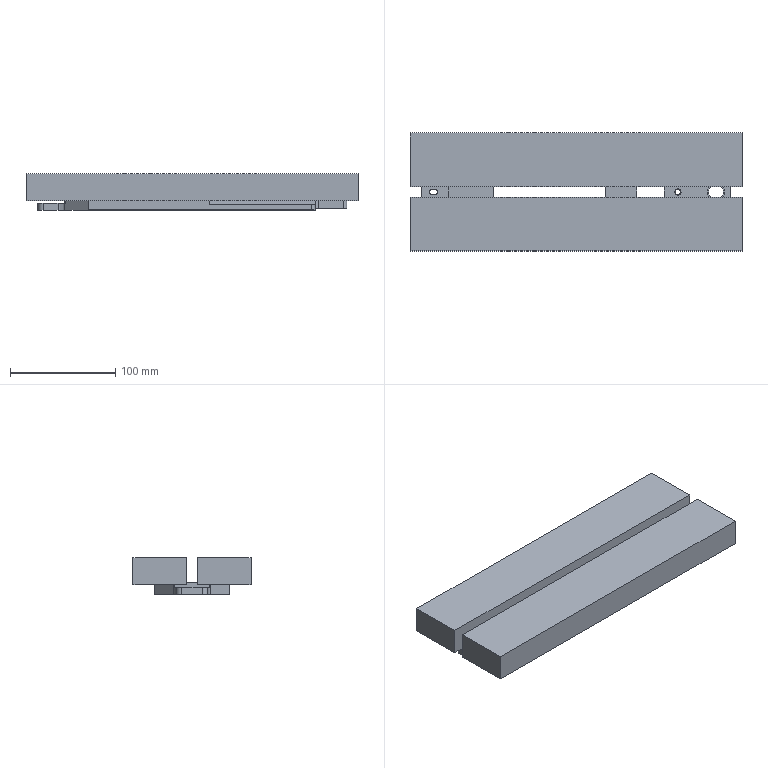NC program | NX | posted with a generic post | part box 315 x 112 x 34.85 mm
Lines 1 to 18 of 11462:
N10 G17 G21 G94 G90
(PLANAR_MILL , TOOL : D100面刀)
N12 T01 M6
N14 G53
N16 G17 G0 G90 X212.5 Y0. S3500 M3
N18 G43 Z20. H1
N20 Z3.
N22 G94 G1 Z0. F800.
N24 X157.5
N26 X-157.5
N28 X-212.5
N30 Z3.
N32 G0 Z20.
N34 M5